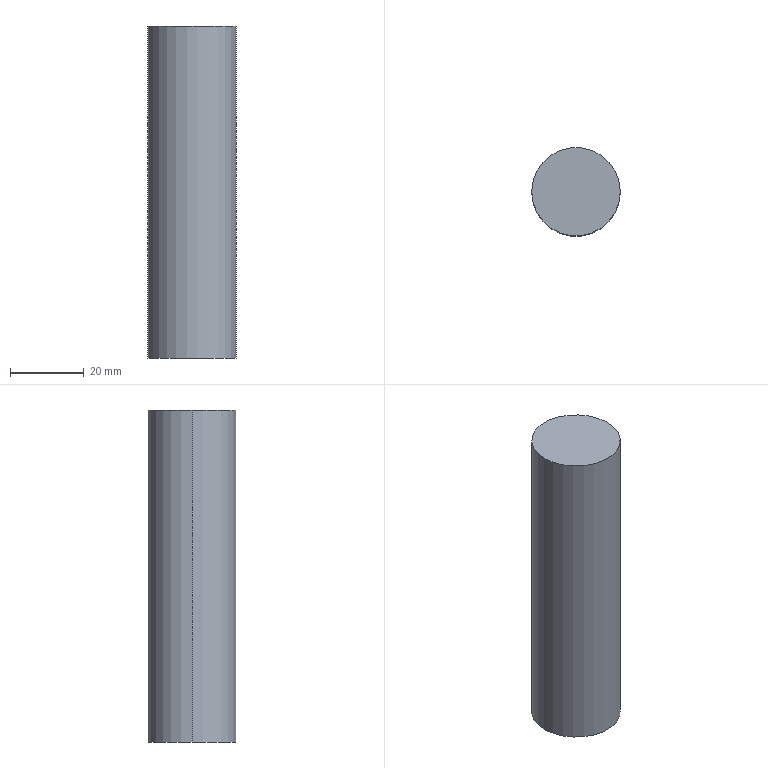Part | SolidWorks | features Extrusion 1 | 1 solid | 4 faces | box 24 x 24 x 90 mm | volume 40715 mm3 | cylinder 2 | plane 2 | commonest cylinder face diameters 24 x2
STEP:
#1=CARTESIAN_POINT('',(12.,0.,90.));
#2=VERTEX_POINT('',#1);
#3=CARTESIAN_POINT('',(-12.,0.,90.));
#4=VERTEX_POINT('',#3);
#5=CARTESIAN_POINT('',(0.,0.,90.));
#6=DIRECTION('',(0.,0.,1.));
#7=DIRECTION('',(1.,0.,0.));
#8=AXIS2_PLACEMENT_3D('',#5,#6,#7);
#9=CIRCLE('',#8,12.);
#10=EDGE_CURVE('',#2,#4,#9,.T.);
#11=ORIENTED_EDGE('',*,*,#10,.F.);
#12=CARTESIAN_POINT('',(12.,0.,0.));
#13=VERTEX_POINT('',#12);
#14=CARTESIAN_POINT('',(12.,0.,90.));
#15=DIRECTION('',(0.,0.,-1.));
#16=VECTOR('',#15,1000.);
#17=LINE('',#14,#16);
#18=EDGE_CURVE('',#2,#13,#17,.T.);
#19=ORIENTED_EDGE('',*,*,#18,.T.);
#20=CARTESIAN_POINT('',(-12.,0.,0.));
#21=VERTEX_POINT('',#20);
#22=CARTESIAN_POINT('',(0.,0.,0.));
#23=DIRECTION('',(0.,0.,1.));
#24=DIRECTION('',(1.,0.,0.));
#25=AXIS2_PLACEMENT_3D('',#22,#23,#24);
#26=CIRCLE('',#25,12.);
#27=EDGE_CURVE('',#13,#21,#26,.T.);
#28=ORIENTED_EDGE('',*,*,#27,.T.);
#29=CARTESIAN_POINT('',(-12.,0.,90.));
#30=DIRECTION('',(0.,0.,-1.));
#31=VECTOR('',#30,1000.);
#32=LINE('',#29,#31);
#33=EDGE_CURVE('',#4,#21,#32,.T.);
#34=ORIENTED_EDGE('',*,*,#33,.F.);
#35=EDGE_LOOP('',(#11,#19,#28,#34));
#36=FACE_OUTER_BOUND('',#35,.T.);
#37=CARTESIAN_POINT('',(0.,0.,90.));
#38=DIRECTION('',(0.,0.,-1.));
#39=DIRECTION('',(-1.,0.,0.));
#40=AXIS2_PLACEMENT_3D('',#37,#38,#39);
#41=CYLINDRICAL_SURFACE('',#40,12.);
#42=ADVANCED_FACE('',(#36),#41,.T.);
#43=ORIENTED_EDGE('',*,*,#18,.F.);
#44=CARTESIAN_POINT('',(0.,0.,90.));
#45=DIRECTION('',(0.,0.,1.));
#46=DIRECTION('',(1.,0.,0.));
#47=AXIS2_PLACEMENT_3D('',#44,#45,#46);
#48=CIRCLE('',#47,12.);
#49=EDGE_CURVE('',#4,#2,#48,.T.);
#50=ORIENTED_EDGE('',*,*,#49,.F.);
#51=ORIENTED_EDGE('',*,*,#33,.T.);
#52=CARTESIAN_POINT('',(0.,0.,0.));
#53=DIRECTION('',(0.,0.,1.));
#54=DIRECTION('',(1.,0.,0.));
#55=AXIS2_PLACEMENT_3D('',#52,#53,#54);
#56=CIRCLE('',#55,12.);
#57=EDGE_CURVE('',#21,#13,#56,.T.);
#58=ORIENTED_EDGE('',*,*,#57,.T.);
#59=EDGE_LOOP('',(#43,#50,#51,#58));
#60=FACE_OUTER_BOUND('',#59,.T.);
#61=CARTESIAN_POINT('',(0.,0.,90.));
#62=DIRECTION('',(0.,0.,-1.));
#63=DIRECTION('',(-1.,0.,0.));
#64=AXIS2_PLACEMENT_3D('',#61,#62,#63);
#65=CYLINDRICAL_SURFACE('',#64,12.);
#66=ADVANCED_FACE('',(#60),#65,.T.);
#67=ORIENTED_EDGE('',*,*,#49,.T.);
#68=ORIENTED_EDGE('',*,*,#10,.T.);
#69=EDGE_LOOP('',(#67,#68));
#70=FACE_OUTER_BOUND('',#69,.T.);
#71=CARTESIAN_POINT('',(0.,0.,90.));
#72=DIRECTION('',(0.,0.,1.));
#73=DIRECTION('',(1.,0.,0.));
#74=AXIS2_PLACEMENT_3D('',#71,#72,#73);
#75=PLANE('',#74);
#76=ADVANCED_FACE('',(#70),#75,.T.);
#77=ORIENTED_EDGE('',*,*,#57,.F.);
#78=ORIENTED_EDGE('',*,*,#27,.F.);
#79=EDGE_LOOP('',(#77,#78));
#80=FACE_OUTER_BOUND('',#79,.T.);
#81=CARTESIAN_POINT('',(0.,0.,0.));
#82=DIRECTION('',(0.,0.,1.));
#83=DIRECTION('',(1.,0.,0.));
#84=AXIS2_PLACEMENT_3D('',#81,#82,#83);
#85=PLANE('',#84);
#86=ADVANCED_FACE('',(#80),#85,.F.);
#87=CLOSED_SHELL('',(#42,#66,#76,#86));
#88=MANIFOLD_SOLID_BREP('',#87);
#89=CARTESIAN_POINT('',(0.,0.,0.));
#90=DIRECTION('',(0.,0.,1.));
#91=DIRECTION('',(1.,0.,0.));
#92=AXIS2_PLACEMENT_3D('',#89,#90,#91);
#93=(LENGTH_UNIT()NAMED_UNIT(*)SI_UNIT(.MILLI.,.METRE.));
#94=UNCERTAINTY_MEASURE_WITH_UNIT(LENGTH_MEASURE(0.00001),#93,'','');
#95=(NAMED_UNIT(*)PLANE_ANGLE_UNIT()SI_UNIT($,.RADIAN.));
#96=(NAMED_UNIT(*)SI_UNIT($,.STERADIAN.)SOLID_ANGLE_UNIT());
#97=(GEOMETRIC_REPRESENTATION_CONTEXT(3)GLOBAL_UNCERTAINTY_ASSIGNED_CONTEXT((#94))GLOBAL_UNIT_ASSIGNED_CONTEXT((#93,#95,#96))REPRESENTATION_CONTEXT('',''));
#98=ADVANCED_BREP_SHAPE_REPRESENTATION('',(#88,#92),#97);